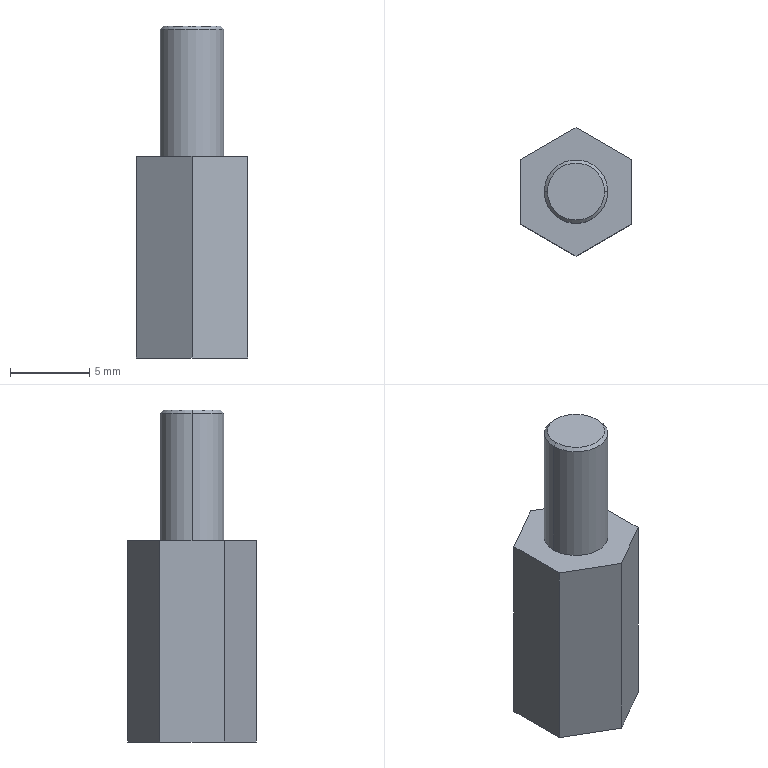Part | STEP file | 49711204_74 | 1 solid | 16 faces | box 7 x 8.09 x 20.9 mm | volume 569.977 mm3 | plane 10 | cylinder 4 | cone 2 | commonest cylinder face diameters 3.2 x2 4 x2
STEP:
#1=CARTESIAN_POINT('',(0.,0.,0.));
#2=DIRECTION('',(0.,0.,1.));
#3=DIRECTION('',(1.,0.,0.));
#4=AXIS2_PLACEMENT_3D('',#1,#2,#3);
#5=CARTESIAN_POINT('',(3.5,-2.024,0.));
#6=VERTEX_POINT('',#5);
#7=CARTESIAN_POINT('',(3.5,2.024,0.));
#8=VERTEX_POINT('',#7);
#9=CARTESIAN_POINT('',(3.5,-2.024,0.));
#10=DIRECTION('',(0.,1.,0.));
#11=VECTOR('',#10,1.);
#12=LINE('',#9,#11);
#13=CARTESIAN_POINT('',(0.,0.,0.));
#14=DIRECTION('',(0.,0.,-1.));
#15=DIRECTION('',(-1.,0.,0.));
#16=AXIS2_PLACEMENT_3D('',#13,#14,#15);
#17=PLANE('',#16);
#18=CARTESIAN_POINT('',(-3.5,-2.024));
#19=DIRECTION('',(0.,1.));
#20=VECTOR('',#19,1.);
#21=LINE('',#18,#20);
#22=(GEOMETRIC_REPRESENTATION_CONTEXT(2)PARAMETRIC_REPRESENTATION_CONTEXT()REPRESENTATION_CONTEXT('',''));
#23=DEFINITIONAL_REPRESENTATION('',(#21),#22);
#24=PCURVE('',#17,#23);
#25=CARTESIAN_POINT('',(3.5,0.,0.));
#26=DIRECTION('',(-1.,0.,0.));
#27=DIRECTION('',(0.,1.,0.));
#28=AXIS2_PLACEMENT_3D('',#25,#26,#27);
#29=PLANE('',#28);
#30=CARTESIAN_POINT('',(-2.024,0.));
#31=DIRECTION('',(1.,0.));
#32=VECTOR('',#31,1.);
#33=LINE('',#30,#32);
#34=(GEOMETRIC_REPRESENTATION_CONTEXT(2)PARAMETRIC_REPRESENTATION_CONTEXT()REPRESENTATION_CONTEXT('',''));
#35=DEFINITIONAL_REPRESENTATION('',(#33),#34);
#36=PCURVE('',#29,#35);
#37=SURFACE_CURVE('',#12,(#24,#36),.PCURVE_S1.);
#38=EDGE_CURVE('',#6,#8,#37,.T.);
#39=ORIENTED_EDGE('',*,*,#38,.F.);
#40=CARTESIAN_POINT('',(0.,-4.045,0.));
#41=VERTEX_POINT('',#40);
#42=CARTESIAN_POINT('',(3.5,-2.024,0.));
#43=DIRECTION('',(-0.866,-0.5,0.));
#44=VECTOR('',#43,1.);
#45=LINE('',#42,#44);
#46=CARTESIAN_POINT('',(-3.5,-2.024));
#47=DIRECTION('',(0.866,-0.5));
#48=VECTOR('',#47,1.);
#49=LINE('',#46,#48);
#50=(GEOMETRIC_REPRESENTATION_CONTEXT(2)PARAMETRIC_REPRESENTATION_CONTEXT()REPRESENTATION_CONTEXT('',''));
#51=DEFINITIONAL_REPRESENTATION('',(#49),#50);
#52=PCURVE('',#17,#51);
#53=CARTESIAN_POINT('',(3.5,-2.024,0.));
#54=DIRECTION('',(0.5,-0.866,0.));
#55=DIRECTION('',(-0.866,-0.5,0.));
#56=AXIS2_PLACEMENT_3D('',#53,#54,#55);
#57=PLANE('',#56);
#58=CARTESIAN_POINT('',(0.,0.));
#59=DIRECTION('',(1.,0.));
#60=VECTOR('',#59,1.);
#61=LINE('',#58,#60);
#62=(GEOMETRIC_REPRESENTATION_CONTEXT(2)PARAMETRIC_REPRESENTATION_CONTEXT()REPRESENTATION_CONTEXT('',''));
#63=DEFINITIONAL_REPRESENTATION('',(#61),#62);
#64=PCURVE('',#57,#63);
#65=SURFACE_CURVE('',#45,(#52,#64),.PCURVE_S1.);
#66=EDGE_CURVE('',#6,#41,#65,.T.);
#67=ORIENTED_EDGE('',*,*,#66,.T.);
#68=CARTESIAN_POINT('',(-3.5,-2.024,0.));
#69=VERTEX_POINT('',#68);
#70=CARTESIAN_POINT('',(-3.5,-2.024,0.));
#71=DIRECTION('',(0.866,-0.5,0.));
#72=VECTOR('',#71,1.);
#73=LINE('',#70,#72);
#74=CARTESIAN_POINT('',(3.5,-2.024));
#75=DIRECTION('',(-0.866,-0.5));
#76=VECTOR('',#75,1.);
#77=LINE('',#74,#76);
#78=(GEOMETRIC_REPRESENTATION_CONTEXT(2)PARAMETRIC_REPRESENTATION_CONTEXT()REPRESENTATION_CONTEXT('',''));
#79=DEFINITIONAL_REPRESENTATION('',(#77),#78);
#80=PCURVE('',#17,#79);
#81=CARTESIAN_POINT('',(-3.5,-2.024,0.));
#82=DIRECTION('',(0.5,0.866,0.));
#83=DIRECTION('',(0.866,-0.5,0.));
#84=AXIS2_PLACEMENT_3D('',#81,#82,#83);
#85=PLANE('',#84);
#86=CARTESIAN_POINT('',(0.,0.));
#87=DIRECTION('',(1.,0.));
#88=VECTOR('',#87,1.);
#89=LINE('',#86,#88);
#90=(GEOMETRIC_REPRESENTATION_CONTEXT(2)PARAMETRIC_REPRESENTATION_CONTEXT()REPRESENTATION_CONTEXT('',''));
#91=DEFINITIONAL_REPRESENTATION('',(#89),#90);
#92=PCURVE('',#85,#91);
#93=SURFACE_CURVE('',#73,(#80,#92),.PCURVE_S1.);
#94=EDGE_CURVE('',#69,#41,#93,.T.);
#95=ORIENTED_EDGE('',*,*,#94,.F.);
#96=CARTESIAN_POINT('',(-3.5,2.024,0.));
#97=VERTEX_POINT('',#96);
#98=CARTESIAN_POINT('',(-3.5,2.024,0.));
#99=DIRECTION('',(0.,-1.,0.));
#100=VECTOR('',#99,1.);
#101=LINE('',#98,#100);
#102=CARTESIAN_POINT('',(3.5,2.024));
#103=DIRECTION('',(0.,-1.));
#104=VECTOR('',#103,1.);
#105=LINE('',#102,#104);
#106=(GEOMETRIC_REPRESENTATION_CONTEXT(2)PARAMETRIC_REPRESENTATION_CONTEXT()REPRESENTATION_CONTEXT('',''));
#107=DEFINITIONAL_REPRESENTATION('',(#105),#106);
#108=PCURVE('',#17,#107);
#109=CARTESIAN_POINT('',(-3.5,0.,0.));
#110=DIRECTION('',(-1.,0.,0.));
#111=DIRECTION('',(0.,1.,0.));
#112=AXIS2_PLACEMENT_3D('',#109,#110,#111);
#113=PLANE('',#112);
#114=CARTESIAN_POINT('',(2.024,0.));
#115=DIRECTION('',(-1.,0.));
#116=VECTOR('',#115,1.);
#117=LINE('',#114,#116);
#118=(GEOMETRIC_REPRESENTATION_CONTEXT(2)PARAMETRIC_REPRESENTATION_CONTEXT()REPRESENTATION_CONTEXT('',''));
#119=DEFINITIONAL_REPRESENTATION('',(#117),#118);
#120=PCURVE('',#113,#119);
#121=SURFACE_CURVE('',#101,(#108,#120),.PCURVE_S1.);
#122=EDGE_CURVE('',#97,#69,#121,.T.);
#123=ORIENTED_EDGE('',*,*,#122,.F.);
#124=CARTESIAN_POINT('',(0.,4.045,0.));
#125=VERTEX_POINT('',#124);
#126=CARTESIAN_POINT('',(-3.5,2.024,0.));
#127=DIRECTION('',(0.866,0.5,0.));
#128=VECTOR('',#127,1.);
#129=LINE('',#126,#128);
#130=CARTESIAN_POINT('',(3.5,2.024));
#131=DIRECTION('',(-0.866,0.5));
#132=VECTOR('',#131,1.);
#133=LINE('',#130,#132);
#134=(GEOMETRIC_REPRESENTATION_CONTEXT(2)PARAMETRIC_REPRESENTATION_CONTEXT()REPRESENTATION_CONTEXT('',''));
#135=DEFINITIONAL_REPRESENTATION('',(#133),#134);
#136=PCURVE('',#17,#135);
#137=CARTESIAN_POINT('',(-3.5,2.024,0.));
#138=DIRECTION('',(-0.5,0.866,0.));
#139=DIRECTION('',(0.866,0.5,0.));
#140=AXIS2_PLACEMENT_3D('',#137,#138,#139);
#141=PLANE('',#140);
#142=CARTESIAN_POINT('',(0.,0.));
#143=DIRECTION('',(1.,0.));
#144=VECTOR('',#143,1.);
#145=LINE('',#142,#144);
#146=(GEOMETRIC_REPRESENTATION_CONTEXT(2)PARAMETRIC_REPRESENTATION_CONTEXT()REPRESENTATION_CONTEXT('',''));
#147=DEFINITIONAL_REPRESENTATION('',(#145),#146);
#148=PCURVE('',#141,#147);
#149=SURFACE_CURVE('',#129,(#136,#148),.PCURVE_S1.);
#150=EDGE_CURVE('',#97,#125,#149,.T.);
#151=ORIENTED_EDGE('',*,*,#150,.T.);
#152=CARTESIAN_POINT('',(3.5,2.024,0.));
#153=DIRECTION('',(-0.866,0.5,0.));
#154=VECTOR('',#153,1.);
#155=LINE('',#152,#154);
#156=CARTESIAN_POINT('',(-3.5,2.024));
#157=DIRECTION('',(0.866,0.5));
#158=VECTOR('',#157,1.);
#159=LINE('',#156,#158);
#160=(GEOMETRIC_REPRESENTATION_CONTEXT(2)PARAMETRIC_REPRESENTATION_CONTEXT()REPRESENTATION_CONTEXT('',''));
#161=DEFINITIONAL_REPRESENTATION('',(#159),#160);
#162=PCURVE('',#17,#161);
#163=CARTESIAN_POINT('',(3.5,2.024,0.));
#164=DIRECTION('',(-0.5,-0.866,0.));
#165=DIRECTION('',(-0.866,0.5,0.));
#166=AXIS2_PLACEMENT_3D('',#163,#164,#165);
#167=PLANE('',#166);
#168=CARTESIAN_POINT('',(0.,0.));
#169=DIRECTION('',(1.,0.));
#170=VECTOR('',#169,1.);
#171=LINE('',#168,#170);
#172=(GEOMETRIC_REPRESENTATION_CONTEXT(2)PARAMETRIC_REPRESENTATION_CONTEXT()REPRESENTATION_CONTEXT('',''));
#173=DEFINITIONAL_REPRESENTATION('',(#171),#172);
#174=PCURVE('',#167,#173);
#175=SURFACE_CURVE('',#155,(#162,#174),.PCURVE_S1.);
#176=EDGE_CURVE('',#8,#125,#175,.T.);
#177=ORIENTED_EDGE('',*,*,#176,.F.);
#178=EDGE_LOOP('',(#39,#67,#95,#123,#151,#177));
#179=FACE_BOUND('',#178,.F.);
#180=CARTESIAN_POINT('',(-2.,0.,0.));
#181=VERTEX_POINT('',#180);
#182=CARTESIAN_POINT('',(2.,0.,0.));
#183=VERTEX_POINT('',#182);
#184=CARTESIAN_POINT('',(0.,0.,0.));
#185=DIRECTION('',(0.,0.,1.));
#186=DIRECTION('',(-1.,0.,0.));
#187=AXIS2_PLACEMENT_3D('',#184,#185,#186);
#188=CIRCLE('',#187,2.);
#189=CARTESIAN_POINT('',(2.,0.));
#190=CARTESIAN_POINT('',(2.,-3.464));
#191=CARTESIAN_POINT('',(-1.,-1.732));
#192=CARTESIAN_POINT('',(-4.,0.));
#193=CARTESIAN_POINT('',(-1.,1.732));
#194=CARTESIAN_POINT('',(2.,3.464));
#195=CARTESIAN_POINT('',(2.,0.));
#196=(BOUNDED_CURVE()B_SPLINE_CURVE(2,(#189,#190,#191,#192,#193,#194,#195),.UNSPECIFIED.,.T.,.F.)B_SPLINE_CURVE_WITH_KNOTS((1,2,2,2,2,1),(-2.094,0.,2.094,4.189,6.283,8.378),.UNSPECIFIED.)CURVE()GEOMETRIC_REPRESENTATION_ITEM()RATIONAL_B_SPLINE_CURVE((1.,0.5,1.,0.5,1.,0.5,1.))REPRESENTATION_ITEM(''));
#197=(GEOMETRIC_REPRESENTATION_CONTEXT(2)PARAMETRIC_REPRESENTATION_CONTEXT()REPRESENTATION_CONTEXT('',''));
#198=DEFINITIONAL_REPRESENTATION('',(#196),#197);
#199=PCURVE('',#17,#198);
#200=CARTESIAN_POINT('',(0.,0.,0.));
#201=DIRECTION('',(0.,0.,1.));
#202=DIRECTION('',(-1.,0.,0.));
#203=AXIS2_PLACEMENT_3D('',#200,#201,#202);
#204=CYLINDRICAL_SURFACE('',#203,2.);
#205=CARTESIAN_POINT('',(0.,0.));
#206=DIRECTION('',(1.,0.));
#207=VECTOR('',#206,1.);
#208=LINE('',#205,#207);
#209=(GEOMETRIC_REPRESENTATION_CONTEXT(2)PARAMETRIC_REPRESENTATION_CONTEXT()REPRESENTATION_CONTEXT('',''));
#210=DEFINITIONAL_REPRESENTATION('',(#208),#209);
#211=PCURVE('',#204,#210);
#212=SURFACE_CURVE('',#188,(#199,#211),.PCURVE_S1.);
#213=EDGE_CURVE('',#181,#183,#212,.T.);
#214=ORIENTED_EDGE('',*,*,#213,.T.);
#215=CARTESIAN_POINT('',(0.,0.,0.));
#216=DIRECTION('',(0.,0.,1.));
#217=DIRECTION('',(1.,0.,0.));
#218=AXIS2_PLACEMENT_3D('',#215,#216,#217);
#219=CIRCLE('',#218,2.);
#220=CARTESIAN_POINT('',(-2.,0.));
#221=CARTESIAN_POINT('',(-2.,3.464));
#222=CARTESIAN_POINT('',(1.,1.732));
#223=CARTESIAN_POINT('',(4.,0.));
#224=CARTESIAN_POINT('',(1.,-1.732));
#225=CARTESIAN_POINT('',(-2.,-3.464));
#226=CARTESIAN_POINT('',(-2.,0.));
#227=(BOUNDED_CURVE()B_SPLINE_CURVE(2,(#220,#221,#222,#223,#224,#225,#226),.UNSPECIFIED.,.T.,.F.)B_SPLINE_CURVE_WITH_KNOTS((1,2,2,2,2,1),(-2.094,0.,2.094,4.189,6.283,8.378),.UNSPECIFIED.)CURVE()GEOMETRIC_REPRESENTATION_ITEM()RATIONAL_B_SPLINE_CURVE((1.,0.5,1.,0.5,1.,0.5,1.))REPRESENTATION_ITEM(''));
#228=(GEOMETRIC_REPRESENTATION_CONTEXT(2)PARAMETRIC_REPRESENTATION_CONTEXT()REPRESENTATION_CONTEXT('',''));
#229=DEFINITIONAL_REPRESENTATION('',(#227),#228);
#230=PCURVE('',#17,#229);
#231=CARTESIAN_POINT('',(0.,0.,0.));
#232=DIRECTION('',(0.,0.,1.));
#233=DIRECTION('',(-1.,0.,0.));
#234=AXIS2_PLACEMENT_3D('',#231,#232,#233);
#235=CYLINDRICAL_SURFACE('',#234,2.);
#236=CARTESIAN_POINT('',(3.142,0.));
#237=DIRECTION('',(1.,0.));
#238=VECTOR('',#237,1.);
#239=LINE('',#236,#238);
#240=(GEOMETRIC_REPRESENTATION_CONTEXT(2)PARAMETRIC_REPRESENTATION_CONTEXT()REPRESENTATION_CONTEXT('',''));
#241=DEFINITIONAL_REPRESENTATION('',(#239),#240);
#242=PCURVE('',#235,#241);
#243=SURFACE_CURVE('',#219,(#230,#242),.PCURVE_S1.);
#244=EDGE_CURVE('',#183,#181,#243,.T.);
#245=ORIENTED_EDGE('',*,*,#244,.T.);
#246=EDGE_LOOP('',(#214,#245));
#247=FACE_BOUND('',#246,.F.);
#248=ADVANCED_FACE('',(#179,#247),#17,.F.);
#249=CARTESIAN_POINT('',(3.5,2.024,-12.7));
#250=VERTEX_POINT('',#249);
#251=CARTESIAN_POINT('',(3.5,-2.024,-12.7));
#252=VERTEX_POINT('',#251);
#253=CARTESIAN_POINT('',(3.5,2.024,-12.7));
#254=DIRECTION('',(0.,-1.,0.));
#255=VECTOR('',#254,1.);
#256=LINE('',#253,#255);
#257=CARTESIAN_POINT('',(2.024,12.7));
#258=DIRECTION('',(-1.,0.));
#259=VECTOR('',#258,1.);
#260=LINE('',#257,#259);
#261=(GEOMETRIC_REPRESENTATION_CONTEXT(2)PARAMETRIC_REPRESENTATION_CONTEXT()REPRESENTATION_CONTEXT('',''));
#262=DEFINITIONAL_REPRESENTATION('',(#260),#261);
#263=PCURVE('',#29,#262);
#264=CARTESIAN_POINT('',(0.,0.,-12.7));
#265=DIRECTION('',(0.,0.,-1.));
#266=DIRECTION('',(-1.,0.,0.));
#267=AXIS2_PLACEMENT_3D('',#264,#265,#266);
#268=PLANE('',#267);
#269=CARTESIAN_POINT('',(-3.5,2.024));
#270=DIRECTION('',(0.,-1.));
#271=VECTOR('',#270,1.);
#272=LINE('',#269,#271);
#273=(GEOMETRIC_REPRESENTATION_CONTEXT(2)PARAMETRIC_REPRESENTATION_CONTEXT()REPRESENTATION_CONTEXT('',''));
#274=DEFINITIONAL_REPRESENTATION('',(#272),#273);
#275=PCURVE('',#268,#274);
#276=SURFACE_CURVE('',#256,(#263,#275),.PCURVE_S1.);
#277=EDGE_CURVE('',#250,#252,#276,.T.);
#278=ORIENTED_EDGE('',*,*,#277,.T.);
#279=CARTESIAN_POINT('',(3.5,-2.024,0.));
#280=DIRECTION('',(0.,0.,-1.));
#281=VECTOR('',#280,1.);
#282=LINE('',#279,#281);
#283=CARTESIAN_POINT('',(-2.024,0.));
#284=DIRECTION('',(0.,1.));
#285=VECTOR('',#284,1.);
#286=LINE('',#283,#285);
#287=(GEOMETRIC_REPRESENTATION_CONTEXT(2)PARAMETRIC_REPRESENTATION_CONTEXT()REPRESENTATION_CONTEXT('',''));
#288=DEFINITIONAL_REPRESENTATION('',(#286),#287);
#289=PCURVE('',#29,#288);
#290=CARTESIAN_POINT('',(0.,0.));
#291=DIRECTION('',(0.,1.));
#292=VECTOR('',#291,1.);
#293=LINE('',#290,#292);
#294=(GEOMETRIC_REPRESENTATION_CONTEXT(2)PARAMETRIC_REPRESENTATION_CONTEXT()REPRESENTATION_CONTEXT('',''));
#295=DEFINITIONAL_REPRESENTATION('',(#293),#294);
#296=PCURVE('',#57,#295);
#297=SURFACE_CURVE('',#282,(#289,#296),.PCURVE_S1.);
#298=EDGE_CURVE('',#6,#252,#297,.T.);
#299=ORIENTED_EDGE('',*,*,#298,.F.);
#300=ORIENTED_EDGE('',*,*,#38,.T.);
#301=CARTESIAN_POINT('',(3.5,2.024,0.));
#302=DIRECTION('',(0.,0.,-1.));
#303=VECTOR('',#302,1.);
#304=LINE('',#301,#303);
#305=CARTESIAN_POINT('',(2.024,0.));
#306=DIRECTION('',(0.,1.));
#307=VECTOR('',#306,1.);
#308=LINE('',#305,#307);
#309=(GEOMETRIC_REPRESENTATION_CONTEXT(2)PARAMETRIC_REPRESENTATION_CONTEXT()REPRESENTATION_CONTEXT('',''));
#310=DEFINITIONAL_REPRESENTATION('',(#308),#309);
#311=PCURVE('',#29,#310);
#312=CARTESIAN_POINT('',(0.,0.));
#313=DIRECTION('',(0.,1.));
#314=VECTOR('',#313,1.);
#315=LINE('',#312,#314);
#316=(GEOMETRIC_REPRESENTATION_CONTEXT(2)PARAMETRIC_REPRESENTATION_CONTEXT()REPRESENTATION_CONTEXT('',''));
#317=DEFINITIONAL_REPRESENTATION('',(#315),#316);
#318=PCURVE('',#167,#317);
#319=SURFACE_CURVE('',#304,(#311,#318),.PCURVE_S1.);
#320=EDGE_CURVE('',#8,#250,#319,.T.);
#321=ORIENTED_EDGE('',*,*,#320,.T.);
#322=EDGE_LOOP('',(#278,#299,#300,#321));
#323=FACE_BOUND('',#322,.F.);
#324=ADVANCED_FACE('',(#323),#29,.F.);
#325=CARTESIAN_POINT('',(-3.5,-2.024,-12.7));
#326=VERTEX_POINT('',#325);
#327=CARTESIAN_POINT('',(0.,-4.045,-12.7));
#328=VERTEX_POINT('',#327);
#329=CARTESIAN_POINT('',(-3.5,-2.024,-12.7));
#330=DIRECTION('',(0.866,-0.5,0.));
#331=VECTOR('',#330,1.);
#332=LINE('',#329,#331);
#333=CARTESIAN_POINT('',(3.5,-2.024));
#334=DIRECTION('',(-0.866,-0.5));
#335=VECTOR('',#334,1.);
#336=LINE('',#333,#335);
#337=(GEOMETRIC_REPRESENTATION_CONTEXT(2)PARAMETRIC_REPRESENTATION_CONTEXT()REPRESENTATION_CONTEXT('',''));
#338=DEFINITIONAL_REPRESENTATION('',(#336),#337);
#339=PCURVE('',#268,#338);
#340=CARTESIAN_POINT('',(0.,12.7));
#341=DIRECTION('',(1.,0.));
#342=VECTOR('',#341,1.);
#343=LINE('',#340,#342);
#344=(GEOMETRIC_REPRESENTATION_CONTEXT(2)PARAMETRIC_REPRESENTATION_CONTEXT()REPRESENTATION_CONTEXT('',''));
#345=DEFINITIONAL_REPRESENTATION('',(#343),#344);
#346=PCURVE('',#85,#345);
#347=SURFACE_CURVE('',#332,(#339,#346),.PCURVE_S1.);
#348=EDGE_CURVE('',#326,#328,#347,.T.);
#349=ORIENTED_EDGE('',*,*,#348,.T.);
#350=CARTESIAN_POINT('',(3.5,-2.024,-12.7));
#351=DIRECTION('',(-0.866,-0.5,0.));
#352=VECTOR('',#351,1.);
#353=LINE('',#350,#352);
#354=CARTESIAN_POINT('',(-3.5,-2.024));
#355=DIRECTION('',(0.866,-0.5));
#356=VECTOR('',#355,1.);
#357=LINE('',#354,#356);
#358=(GEOMETRIC_REPRESENTATION_CONTEXT(2)PARAMETRIC_REPRESENTATION_CONTEXT()REPRESENTATION_CONTEXT('',''));
#359=DEFINITIONAL_REPRESENTATION('',(#357),#358);
#360=PCURVE('',#268,#359);
#361=CARTESIAN_POINT('',(0.,12.7));
#362=DIRECTION('',(1.,0.));
#363=VECTOR('',#362,1.);
#364=LINE('',#361,#363);
#365=(GEOMETRIC_REPRESENTATION_CONTEXT(2)PARAMETRIC_REPRESENTATION_CONTEXT()REPRESENTATION_CONTEXT('',''));
#366=DEFINITIONAL_REPRESENTATION('',(#364),#365);
#367=PCURVE('',#57,#366);
#368=SURFACE_CURVE('',#353,(#360,#367),.PCURVE_S1.);
#369=EDGE_CURVE('',#252,#328,#368,.T.);
#370=ORIENTED_EDGE('',*,*,#369,.F.);
#371=ORIENTED_EDGE('',*,*,#277,.F.);
#372=CARTESIAN_POINT('',(0.,4.045,-12.7));
#373=VERTEX_POINT('',#372);
#374=CARTESIAN_POINT('',(3.5,2.024,-12.7));
#375=DIRECTION('',(-0.866,0.5,0.));
#376=VECTOR('',#375,1.);
#377=LINE('',#374,#376);
#378=CARTESIAN_POINT('',(-3.5,2.024));
#379=DIRECTION('',(0.866,0.5));
#380=VECTOR('',#379,1.);
#381=LINE('',#378,#380);
#382=(GEOMETRIC_REPRESENTATION_CONTEXT(2)PARAMETRIC_REPRESENTATION_CONTEXT()REPRESENTATION_CONTEXT('',''));
#383=DEFINITIONAL_REPRESENTATION('',(#381),#382);
#384=PCURVE('',#268,#383);
#385=CARTESIAN_POINT('',(0.,12.7));
#386=DIRECTION('',(1.,0.));
#387=VECTOR('',#386,1.);
#388=LINE('',#385,#387);
#389=(GEOMETRIC_REPRESENTATION_CONTEXT(2)PARAMETRIC_REPRESENTATION_CONTEXT()REPRESENTATION_CONTEXT('',''));
#390=DEFINITIONAL_REPRESENTATION('',(#388),#389);
#391=PCURVE('',#167,#390);
#392=SURFACE_CURVE('',#377,(#384,#391),.PCURVE_S1.);
#393=EDGE_CURVE('',#250,#373,#392,.T.);
#394=ORIENTED_EDGE('',*,*,#393,.T.);
#395=CARTESIAN_POINT('',(-3.5,2.024,-12.7));
#396=VERTEX_POINT('',#395);
#397=CARTESIAN_POINT('',(-3.5,2.024,-12.7));
#398=DIRECTION('',(0.866,0.5,0.));
#399=VECTOR('',#398,1.);
#400=LINE('',#397,#399);
#401=CARTESIAN_POINT('',(3.5,2.024));
#402=DIRECTION('',(-0.866,0.5));
#403=VECTOR('',#402,1.);
#404=LINE('',#401,#403);
#405=(GEOMETRIC_REPRESENTATION_CONTEXT(2)PARAMETRIC_REPRESENTATION_CONTEXT()REPRESENTATION_CONTEXT('',''));
#406=DEFINITIONAL_REPRESENTATION('',(#404),#405);
#407=PCURVE('',#268,#406);
#408=CARTESIAN_POINT('',(0.,12.7));
#409=DIRECTION('',(1.,0.));
#410=VECTOR('',#409,1.);
#411=LINE('',#408,#410);
#412=(GEOMETRIC_REPRESENTATION_CONTEXT(2)PARAMETRIC_REPRESENTATION_CONTEXT()REPRESENTATION_CONTEXT('',''));
#413=DEFINITIONAL_REPRESENTATION('',(#411),#412);
#414=PCURVE('',#141,#413);
#415=SURFACE_CURVE('',#400,(#407,#414),.PCURVE_S1.);
#416=EDGE_CURVE('',#396,#373,#415,.T.);
#417=ORIENTED_EDGE('',*,*,#416,.F.);
#418=CARTESIAN_POINT('',(-3.5,-2.024,-12.7));
#419=DIRECTION('',(0.,1.,0.));
#420=VECTOR('',#419,1.);
#421=LINE('',#418,#420);
#422=CARTESIAN_POINT('',(3.5,-2.024));
#423=DIRECTION('',(0.,1.));
#424=VECTOR('',#423,1.);
#425=LINE('',#422,#424);
#426=(GEOMETRIC_REPRESENTATION_CONTEXT(2)PARAMETRIC_REPRESENTATION_CONTEXT()REPRESENTATION_CONTEXT('',''));
#427=DEFINITIONAL_REPRESENTATION('',(#425),#426);
#428=PCURVE('',#268,#427);
#429=CARTESIAN_POINT('',(-2.024,12.7));
#430=DIRECTION('',(1.,0.));
#431=VECTOR('',#430,1.);
#432=LINE('',#429,#431);
#433=(GEOMETRIC_REPRESENTATION_CONTEXT(2)PARAMETRIC_REPRESENTATION_CONTEXT()REPRESENTATION_CONTEXT('',''));
#434=DEFINITIONAL_REPRESENTATION('',(#432),#433);
#435=PCURVE('',#113,#434);
#436=SURFACE_CURVE('',#421,(#428,#435),.PCURVE_S1.);
#437=EDGE_CURVE('',#326,#396,#436,.T.);
#438=ORIENTED_EDGE('',*,*,#437,.F.);
#439=EDGE_LOOP('',(#349,#370,#371,#394,#417,#438));
#440=FACE_BOUND('',#439,.F.);
#441=CARTESIAN_POINT('',(1.6,0.,-12.7));
#442=VERTEX_POINT('',#441);
#443=CARTESIAN_POINT('',(-1.6,0.,-12.7));
#444=VERTEX_POINT('',#443);
#445=CARTESIAN_POINT('',(0.,0.,-12.7));
#446=DIRECTION('',(0.,0.,-1.));
#447=DIRECTION('',(1.,0.,0.));
#448=AXIS2_PLACEMENT_3D('',#445,#446,#447);
#449=CIRCLE('',#448,1.6);
#450=CARTESIAN_POINT('',(0.,0.));
#451=DIRECTION('',(-1.,0.));
#452=AXIS2_PLACEMENT_2D('',#450,#451);
#453=CIRCLE('',#452,1.6);
#454=(GEOMETRIC_REPRESENTATION_CONTEXT(2)PARAMETRIC_REPRESENTATION_CONTEXT()REPRESENTATION_CONTEXT('',''));
#455=DEFINITIONAL_REPRESENTATION('',(#453),#454);
#456=PCURVE('',#268,#455);
#457=CARTESIAN_POINT('',(0.,0.,-12.7));
#458=DIRECTION('',(0.,0.,-1.));
#459=DIRECTION('',(1.,0.,0.));
#460=AXIS2_PLACEMENT_3D('',#457,#458,#459);
#461=CYLINDRICAL_SURFACE('',#460,1.6);
#462=CARTESIAN_POINT('',(0.,0.));
#463=DIRECTION('',(1.,0.));
#464=VECTOR('',#463,1.);
#465=LINE('',#462,#464);
#466=(GEOMETRIC_REPRESENTATION_CONTEXT(2)PARAMETRIC_REPRESENTATION_CONTEXT()REPRESENTATION_CONTEXT('',''));
#467=DEFINITIONAL_REPRESENTATION('',(#465),#466);
#468=PCURVE('',#461,#467);
#469=SURFACE_CURVE('',#449,(#456,#468),.PCURVE_S1.);
#470=EDGE_CURVE('',#442,#444,#469,.T.);
#471=ORIENTED_EDGE('',*,*,#470,.T.);
#472=CARTESIAN_POINT('',(0.,0.,-12.7));
#473=DIRECTION('',(0.,0.,-1.));
#474=DIRECTION('',(-1.,0.,0.));
#475=AXIS2_PLACEMENT_3D('',#472,#473,#474);
#476=CIRCLE('',#475,1.6);
#477=CARTESIAN_POINT('',(0.,0.));
#478=DIRECTION('',(1.,0.));
#479=AXIS2_PLACEMENT_2D('',#477,#478);
#480=CIRCLE('',#479,1.6);
#481=(GEOMETRIC_REPRESENTATION_CONTEXT(2)PARAMETRIC_REPRESENTATION_CONTEXT()REPRESENTATION_CONTEXT('',''));
#482=DEFINITIONAL_REPRESENTATION('',(#480),#481);
#483=PCURVE('',#268,#482);
#484=CARTESIAN_POINT('',(0.,0.,-12.7));
#485=DIRECTION('',(0.,0.,-1.));
#486=DIRECTION('',(1.,0.,0.));
#487=AXIS2_PLACEMENT_3D('',#484,#485,#486);
#488=CYLINDRICAL_SURFACE('',#487,1.6);
#489=CARTESIAN_POINT('',(3.142,0.));
#490=DIRECTION('',(1.,0.));
#491=VECTOR('',#490,1.);
#492=LINE('',#489,#491);
#493=(GEOMETRIC_REPRESENTATION_CONTEXT(2)PARAMETRIC_REPRESENTATION_CONTEXT()REPRESENTATION_CONTEXT('',''));
#494=DEFINITIONAL_REPRESENTATION('',(#492),#493);
#495=PCURVE('',#488,#494);
#496=SURFACE_CURVE('',#476,(#483,#495),.PCURVE_S1.);
#497=EDGE_CURVE('',#444,#442,#496,.T.);
#498=ORIENTED_EDGE('',*,*,#497,.T.);
#499=EDGE_LOOP('',(#471,#498));
#500=FACE_BOUND('',#499,.F.);
#501=ADVANCED_FACE('',(#440,#500),#268,.T.);
#502=CARTESIAN_POINT('',(0.,-4.045,0.));
#503=DIRECTION('',(0.,0.,-1.));
#504=VECTOR('',#503,1.);
#505=LINE('',#502,#504);
#506=CARTESIAN_POINT('',(4.041,0.));
#507=DIRECTION('',(0.,1.));
#508=VECTOR('',#507,1.);
#509=LINE('',#506,#508);
#510=(GEOMETRIC_REPRESENTATION_CONTEXT(2)PARAMETRIC_REPRESENTATION_CONTEXT()REPRESENTATION_CONTEXT('',''));
#511=DEFINITIONAL_REPRESENTATION('',(#509),#510);
#512=PCURVE('',#85,#511);
#513=CARTESIAN_POINT('',(4.041,0.));
#514=DIRECTION('',(0.,1.));
#515=VECTOR('',#514,1.);
#516=LINE('',#513,#515);
#517=(GEOMETRIC_REPRESENTATION_CONTEXT(2)PARAMETRIC_REPRESENTATION_CONTEXT()REPRESENTATION_CONTEXT('',''));
#518=DEFINITIONAL_REPRESENTATION('',(#516),#517);
#519=PCURVE('',#57,#518);
#520=SURFACE_CURVE('',#505,(#512,#519),.PCURVE_S1.);
#521=EDGE_CURVE('',#41,#328,#520,.T.);
#522=ORIENTED_EDGE('',*,*,#521,.T.);
#523=ORIENTED_EDGE('',*,*,#348,.F.);
#524=CARTESIAN_POINT('',(-3.5,-2.024,0.));
#525=DIRECTION('',(0.,0.,-1.));
#526=VECTOR('',#525,1.);
#527=LINE('',#524,#526);
#528=CARTESIAN_POINT('',(0.,0.));
#529=DIRECTION('',(0.,1.));
#530=VECTOR('',#529,1.);
#531=LINE('',#528,#530);
#532=(GEOMETRIC_REPRESENTATION_CONTEXT(2)PARAMETRIC_REPRESENTATION_CONTEXT()REPRESENTATION_CONTEXT('',''));
#533=DEFINITIONAL_REPRESENTATION('',(#531),#532);
#534=PCURVE('',#85,#533);
#535=CARTESIAN_POINT('',(-2.024,0.));
#536=DIRECTION('',(0.,1.));
#537=VECTOR('',#536,1.);
#538=LINE('',#535,#537);
#539=(GEOMETRIC_REPRESENTATION_CONTEXT(2)PARAMETRIC_REPRESENTATION_CONTEXT()REPRESENTATION_CONTEXT('',''));
#540=DEFINITIONAL_REPRESENTATION('',(#538),#539);
#541=PCURVE('',#113,#540);
#542=SURFACE_CURVE('',#527,(#534,#541),.PCURVE_S1.);
#543=EDGE_CURVE('',#69,#326,#542,.T.);
#544=ORIENTED_EDGE('',*,*,#543,.F.);
#545=ORIENTED_EDGE('',*,*,#94,.T.);
#546=EDGE_LOOP('',(#522,#523,#544,#545));
#547=FACE_BOUND('',#546,.F.);
#548=ADVANCED_FACE('',(#547),#85,.F.);
#549=ORIENTED_EDGE('',*,*,#521,.F.);
#550=ORIENTED_EDGE('',*,*,#66,.F.);
#551=ORIENTED_EDGE('',*,*,#298,.T.);
#552=ORIENTED_EDGE('',*,*,#369,.T.);
#553=EDGE_LOOP('',(#549,#550,#551,#552));
#554=FACE_BOUND('',#553,.F.);
#555=ADVANCED_FACE('',(#554),#57,.T.);
#556=ORIENTED_EDGE('',*,*,#122,.T.);
#557=ORIENTED_EDGE('',*,*,#543,.T.);
#558=ORIENTED_EDGE('',*,*,#437,.T.);
#559=CARTESIAN_POINT('',(-3.5,2.024,0.));
#560=DIRECTION('',(0.,0.,-1.));
#561=VECTOR('',#560,1.);
#562=LINE('',#559,#561);
#563=CARTESIAN_POINT('',(2.024,0.));
#564=DIRECTION('',(0.,1.));
#565=VECTOR('',#564,1.);
#566=LINE('',#563,#565);
#567=(GEOMETRIC_REPRESENTATION_CONTEXT(2)PARAMETRIC_REPRESENTATION_CONTEXT()REPRESENTATION_CONTEXT('',''));
#568=DEFINITIONAL_REPRESENTATION('',(#566),#567);
#569=PCURVE('',#113,#568);
#570=CARTESIAN_POINT('',(0.,0.));
#571=DIRECTION('',(0.,1.));
#572=VECTOR('',#571,1.);
#573=LINE('',#570,#572);
#574=(GEOMETRIC_REPRESENTATION_CONTEXT(2)PARAMETRIC_REPRESENTATION_CONTEXT()REPRESENTATION_CONTEXT('',''));
#575=DEFINITIONAL_REPRESENTATION('',(#573),#574);
#576=PCURVE('',#141,#575);
#577=SURFACE_CURVE('',#562,(#569,#576),.PCURVE_S1.);
#578=EDGE_CURVE('',#97,#396,#577,.T.);
#579=ORIENTED_EDGE('',*,*,#578,.F.);
#580=EDGE_LOOP('',(#556,#557,#558,#579));
#581=FACE_BOUND('',#580,.F.);
#582=ADVANCED_FACE('',(#581),#113,.T.);
#583=CARTESIAN_POINT('',(0.,4.045,0.));
#584=DIRECTION('',(0.,0.,-1.));
#585=VECTOR('',#584,1.);
#586=LINE('',#583,#585);
#587=CARTESIAN_POINT('',(4.041,0.));
#588=DIRECTION('',(0.,1.));
#589=VECTOR('',#588,1.);
#590=LINE('',#587,#589);
#591=(GEOMETRIC_REPRESENTATION_CONTEXT(2)PARAMETRIC_REPRESENTATION_CONTEXT()REPRESENTATION_CONTEXT('',''));
#592=DEFINITIONAL_REPRESENTATION('',(#590),#591);
#593=PCURVE('',#141,#592);
#594=CARTESIAN_POINT('',(4.041,0.));
#595=DIRECTION('',(0.,1.));
#596=VECTOR('',#595,1.);
#597=LINE('',#594,#596);
#598=(GEOMETRIC_REPRESENTATION_CONTEXT(2)PARAMETRIC_REPRESENTATION_CONTEXT()REPRESENTATION_CONTEXT('',''));
#599=DEFINITIONAL_REPRESENTATION('',(#597),#598);
#600=PCURVE('',#167,#599);
#601=SURFACE_CURVE('',#586,(#593,#600),.PCURVE_S1.);
#602=EDGE_CURVE('',#125,#373,#601,.T.);
#603=ORIENTED_EDGE('',*,*,#602,.F.);
#604=ORIENTED_EDGE('',*,*,#150,.F.);
#605=ORIENTED_EDGE('',*,*,#578,.T.);
#606=ORIENTED_EDGE('',*,*,#416,.T.);
#607=EDGE_LOOP('',(#603,#604,#605,#606));
#608=FACE_BOUND('',#607,.F.);
#609=ADVANCED_FACE('',(#608),#141,.T.);
#610=ORIENTED_EDGE('',*,*,#602,.T.);
#611=ORIENTED_EDGE('',*,*,#393,.F.);
#612=ORIENTED_EDGE('',*,*,#320,.F.);
#613=ORIENTED_EDGE('',*,*,#176,.T.);
#614=EDGE_LOOP('',(#610,#611,#612,#613));
#615=FACE_BOUND('',#614,.F.);
#616=ADVANCED_FACE('',(#615),#167,.F.);
#617=ORIENTED_EDGE('',*,*,#470,.F.);
#618=CARTESIAN_POINT('',(1.6,0.,-3.7));
#619=VERTEX_POINT('',#618);
#620=CARTESIAN_POINT('',(1.6,0.,-12.7));
#621=DIRECTION('',(0.,0.,1.));
#622=VECTOR('',#621,1.);
#623=LINE('',#620,#622);
#624=CARTESIAN_POINT('',(0.,0.));
#625=DIRECTION('',(0.,-1.));
#626=VECTOR('',#625,1.);
#627=LINE('',#624,#626);
#628=(GEOMETRIC_REPRESENTATION_CONTEXT(2)PARAMETRIC_REPRESENTATION_CONTEXT()REPRESENTATION_CONTEXT('',''));
#629=DEFINITIONAL_REPRESENTATION('',(#627),#628);
#630=PCURVE('',#461,#629);
#631=CARTESIAN_POINT('',(6.283,0.));
#632=DIRECTION('',(0.,-1.));
#633=VECTOR('',#632,1.);
#634=LINE('',#631,#633);
#635=(GEOMETRIC_REPRESENTATION_CONTEXT(2)PARAMETRIC_REPRESENTATION_CONTEXT()REPRESENTATION_CONTEXT('',''));
#636=DEFINITIONAL_REPRESENTATION('',(#634),#635);
#637=PCURVE('',#488,#636);
#638=SURFACE_CURVE('',#623,(#630,#637),.PCURVE_S1.);
#639=EDGE_CURVE('',#442,#619,#638,.T.);
#640=ORIENTED_EDGE('',*,*,#639,.T.);
#641=CARTESIAN_POINT('',(-1.6,0.,-3.7));
#642=VERTEX_POINT('',#641);
#643=CARTESIAN_POINT('',(0.,0.,-3.7));
#644=DIRECTION('',(0.,0.,-1.));
#645=DIRECTION('',(1.,0.,0.));
#646=AXIS2_PLACEMENT_3D('',#643,#644,#645);
#647=CIRCLE('',#646,1.6);
#648=CARTESIAN_POINT('',(0.,-9.));
#649=DIRECTION('',(1.,0.));
#650=VECTOR('',#649,1.);
#651=LINE('',#648,#650);
#652=(GEOMETRIC_REPRESENTATION_CONTEXT(2)PARAMETRIC_REPRESENTATION_CONTEXT()REPRESENTATION_CONTEXT('',''));
#653=DEFINITIONAL_REPRESENTATION('',(#651),#652);
#654=PCURVE('',#461,#653);
#655=CARTESIAN_POINT('',(0.,0.,-3.7));
#656=DIRECTION('',(0.,0.,-1.));
#657=DIRECTION('',(1.,0.,0.));
#658=AXIS2_PLACEMENT_3D('',#655,#656,#657);
#659=PLANE('',#658);
#660=CARTESIAN_POINT('',(0.,0.));
#661=DIRECTION('',(1.,0.));
#662=AXIS2_PLACEMENT_2D('',#660,#661);
#663=CIRCLE('',#662,1.6);
#664=(GEOMETRIC_REPRESENTATION_CONTEXT(2)PARAMETRIC_REPRESENTATION_CONTEXT()REPRESENTATION_CONTEXT('',''));
#665=DEFINITIONAL_REPRESENTATION('',(#663),#664);
#666=PCURVE('',#659,#665);
#667=SURFACE_CURVE('',#647,(#654,#666),.PCURVE_S1.);
#668=EDGE_CURVE('',#619,#642,#667,.T.);
#669=ORIENTED_EDGE('',*,*,#668,.T.);
#670=CARTESIAN_POINT('',(-1.6,0.,-12.7));
#671=DIRECTION('',(0.,0.,1.));
#672=VECTOR('',#671,1.);
#673=LINE('',#670,#672);
#674=CARTESIAN_POINT('',(3.142,0.));
#675=DIRECTION('',(0.,-1.));
#676=VECTOR('',#675,1.);
#677=LINE('',#674,#676);
#678=(GEOMETRIC_REPRESENTATION_CONTEXT(2)PARAMETRIC_REPRESENTATION_CONTEXT()REPRESENTATION_CONTEXT('',''));
#679=DEFINITIONAL_REPRESENTATION('',(#677),#678);
#680=PCURVE('',#461,#679);
#681=CARTESIAN_POINT('',(3.142,0.));
#682=DIRECTION('',(0.,-1.));
#683=VECTOR('',#682,1.);
#684=LINE('',#681,#683);
#685=(GEOMETRIC_REPRESENTATION_CONTEXT(2)PARAMETRIC_REPRESENTATION_CONTEXT()REPRESENTATION_CONTEXT('',''));
#686=DEFINITIONAL_REPRESENTATION('',(#684),#685);
#687=PCURVE('',#488,#686);
#688=SURFACE_CURVE('',#673,(#680,#687),.PCURVE_S1.);
#689=EDGE_CURVE('',#444,#642,#688,.T.);
#690=ORIENTED_EDGE('',*,*,#689,.F.);
#691=EDGE_LOOP('',(#617,#640,#669,#690));
#692=FACE_BOUND('',#691,.F.);
#693=ADVANCED_FACE('',(#692),#461,.F.);
#694=ORIENTED_EDGE('',*,*,#497,.F.);
#695=ORIENTED_EDGE('',*,*,#689,.T.);
#696=CARTESIAN_POINT('',(0.,0.,-3.7));
#697=DIRECTION('',(0.,0.,-1.));
#698=DIRECTION('',(-1.,0.,0.));
#699=AXIS2_PLACEMENT_3D('',#696,#697,#698);
#700=CIRCLE('',#699,1.6);
#701=CARTESIAN_POINT('',(3.142,-9.));
#702=DIRECTION('',(1.,0.));
#703=VECTOR('',#702,1.);
#704=LINE('',#701,#703);
#705=(GEOMETRIC_REPRESENTATION_CONTEXT(2)PARAMETRIC_REPRESENTATION_CONTEXT()REPRESENTATION_CONTEXT('',''));
#706=DEFINITIONAL_REPRESENTATION('',(#704),#705);
#707=PCURVE('',#488,#706);
#708=CARTESIAN_POINT('',(0.,0.));
#709=DIRECTION('',(-1.,0.));
#710=AXIS2_PLACEMENT_2D('',#708,#709);
#711=CIRCLE('',#710,1.6);
#712=(GEOMETRIC_REPRESENTATION_CONTEXT(2)PARAMETRIC_REPRESENTATION_CONTEXT()REPRESENTATION_CONTEXT('',''));
#713=DEFINITIONAL_REPRESENTATION('',(#711),#712);
#714=PCURVE('',#659,#713);
#715=SURFACE_CURVE('',#700,(#707,#714),.PCURVE_S1.);
#716=EDGE_CURVE('',#642,#619,#715,.T.);
#717=ORIENTED_EDGE('',*,*,#716,.T.);
#718=ORIENTED_EDGE('',*,*,#639,.F.);
#719=EDGE_LOOP('',(#694,#695,#717,#718));
#720=FACE_BOUND('',#719,.F.);
#721=ADVANCED_FACE('',(#720),#488,.F.);
#722=ORIENTED_EDGE('',*,*,#668,.F.);
#723=ORIENTED_EDGE('',*,*,#716,.F.);
#724=EDGE_LOOP('',(#722,#723));
#725=FACE_BOUND('',#724,.F.);
#726=ADVANCED_FACE('',(#725),#659,.T.);
#727=CARTESIAN_POINT('',(2.,0.,8.));
#728=VERTEX_POINT('',#727);
#729=CARTESIAN_POINT('',(2.,0.,0.));
#730=DIRECTION('',(0.,0.,1.));
#731=VECTOR('',#730,1.);
#732=LINE('',#729,#731);
#733=CARTESIAN_POINT('',(3.142,0.));
#734=DIRECTION('',(0.,1.));
#735=VECTOR('',#734,1.);
#736=LINE('',#733,#735);
#737=(GEOMETRIC_REPRESENTATION_CONTEXT(2)PARAMETRIC_REPRESENTATION_CONTEXT()REPRESENTATION_CONTEXT('',''));
#738=DEFINITIONAL_REPRESENTATION('',(#736),#737);
#739=PCURVE('',#204,#738);
#740=CARTESIAN_POINT('',(3.142,0.));
#741=DIRECTION('',(0.,1.));
#742=VECTOR('',#741,1.);
#743=LINE('',#740,#742);
#744=(GEOMETRIC_REPRESENTATION_CONTEXT(2)PARAMETRIC_REPRESENTATION_CONTEXT()REPRESENTATION_CONTEXT('',''));
#745=DEFINITIONAL_REPRESENTATION('',(#743),#744);
#746=PCURVE('',#235,#745);
#747=SURFACE_CURVE('',#732,(#739,#746),.PCURVE_S1.);
#748=EDGE_CURVE('',#183,#728,#747,.T.);
#749=ORIENTED_EDGE('',*,*,#748,.T.);
#750=CARTESIAN_POINT('',(-2.,0.,8.));
#751=VERTEX_POINT('',#750);
#752=CARTESIAN_POINT('',(0.,0.,8.));
#753=DIRECTION('',(0.,0.,1.));
#754=DIRECTION('',(-1.,0.,0.));
#755=AXIS2_PLACEMENT_3D('',#752,#753,#754);
#756=CIRCLE('',#755,2.);
#757=CARTESIAN_POINT('',(0.,8.));
#758=DIRECTION('',(1.,0.));
#759=VECTOR('',#758,1.);
#760=LINE('',#757,#759);
#761=(GEOMETRIC_REPRESENTATION_CONTEXT(2)PARAMETRIC_REPRESENTATION_CONTEXT()REPRESENTATION_CONTEXT('',''));
#762=DEFINITIONAL_REPRESENTATION('',(#760),#761);
#763=PCURVE('',#204,#762);
#764=CARTESIAN_POINT('',(0.,0.,8.1));
#765=DIRECTION('',(0.,0.,-1.));
#766=DIRECTION('',(1.,0.,0.));
#767=AXIS2_PLACEMENT_3D('',#764,#765,#766);
#768=CONICAL_SURFACE('',#767,1.9,0.7854);
#769=CARTESIAN_POINT('',(3.142,0.1));
#770=DIRECTION('',(-1.,0.));
#771=VECTOR('',#770,1.);
#772=LINE('',#769,#771);
#773=(GEOMETRIC_REPRESENTATION_CONTEXT(2)PARAMETRIC_REPRESENTATION_CONTEXT()REPRESENTATION_CONTEXT('',''));
#774=DEFINITIONAL_REPRESENTATION('',(#772),#773);
#775=PCURVE('',#768,#774);
#776=SURFACE_CURVE('',#756,(#763,#775),.PCURVE_S1.);
#777=EDGE_CURVE('',#751,#728,#776,.T.);
#778=ORIENTED_EDGE('',*,*,#777,.F.);
#779=CARTESIAN_POINT('',(-2.,0.,0.));
#780=DIRECTION('',(0.,0.,1.));
#781=VECTOR('',#780,1.);
#782=LINE('',#779,#781);
#783=CARTESIAN_POINT('',(0.,0.));
#784=DIRECTION('',(0.,1.));
#785=VECTOR('',#784,1.);
#786=LINE('',#783,#785);
#787=(GEOMETRIC_REPRESENTATION_CONTEXT(2)PARAMETRIC_REPRESENTATION_CONTEXT()REPRESENTATION_CONTEXT('',''));
#788=DEFINITIONAL_REPRESENTATION('',(#786),#787);
#789=PCURVE('',#204,#788);
#790=CARTESIAN_POINT('',(6.283,0.));
#791=DIRECTION('',(0.,1.));
#792=VECTOR('',#791,1.);
#793=LINE('',#790,#792);
#794=(GEOMETRIC_REPRESENTATION_CONTEXT(2)PARAMETRIC_REPRESENTATION_CONTEXT()REPRESENTATION_CONTEXT('',''));
#795=DEFINITIONAL_REPRESENTATION('',(#793),#794);
#796=PCURVE('',#235,#795);
#797=SURFACE_CURVE('',#782,(#789,#796),.PCURVE_S1.);
#798=EDGE_CURVE('',#181,#751,#797,.T.);
#799=ORIENTED_EDGE('',*,*,#798,.F.);
#800=ORIENTED_EDGE('',*,*,#213,.T.);
#801=EDGE_LOOP('',(#749,#778,#799,#800));
#802=FACE_BOUND('',#801,.T.);
#803=ADVANCED_FACE('',(#802),#204,.T.);
#804=ORIENTED_EDGE('',*,*,#798,.T.);
#805=CARTESIAN_POINT('',(0.,0.,8.));
#806=DIRECTION('',(0.,0.,1.));
#807=DIRECTION('',(1.,0.,0.));
#808=AXIS2_PLACEMENT_3D('',#805,#806,#807);
#809=CIRCLE('',#808,2.);
#810=CARTESIAN_POINT('',(3.142,8.));
#811=DIRECTION('',(1.,0.));
#812=VECTOR('',#811,1.);
#813=LINE('',#810,#812);
#814=(GEOMETRIC_REPRESENTATION_CONTEXT(2)PARAMETRIC_REPRESENTATION_CONTEXT()REPRESENTATION_CONTEXT('',''));
#815=DEFINITIONAL_REPRESENTATION('',(#813),#814);
#816=PCURVE('',#235,#815);
#817=CARTESIAN_POINT('',(0.,0.,8.1));
#818=DIRECTION('',(0.,0.,-1.));
#819=DIRECTION('',(1.,0.,0.));
#820=AXIS2_PLACEMENT_3D('',#817,#818,#819);
#821=CONICAL_SURFACE('',#820,1.9,0.7854);
#822=CARTESIAN_POINT('',(6.283,0.1));
#823=DIRECTION('',(-1.,0.));
#824=VECTOR('',#823,1.);
#825=LINE('',#822,#824);
#826=(GEOMETRIC_REPRESENTATION_CONTEXT(2)PARAMETRIC_REPRESENTATION_CONTEXT()REPRESENTATION_CONTEXT('',''));
#827=DEFINITIONAL_REPRESENTATION('',(#825),#826);
#828=PCURVE('',#821,#827);
#829=SURFACE_CURVE('',#809,(#816,#828),.PCURVE_S1.);
#830=EDGE_CURVE('',#728,#751,#829,.T.);
#831=ORIENTED_EDGE('',*,*,#830,.F.);
#832=ORIENTED_EDGE('',*,*,#748,.F.);
#833=ORIENTED_EDGE('',*,*,#244,.T.);
#834=EDGE_LOOP('',(#804,#831,#832,#833));
#835=FACE_BOUND('',#834,.T.);
#836=ADVANCED_FACE('',(#835),#235,.T.);
#837=CARTESIAN_POINT('',(1.8,0.,8.2));
#838=VERTEX_POINT('',#837);
#839=CARTESIAN_POINT('',(1.8,0.,8.2));
#840=DIRECTION('',(0.7071,0.,-0.7071));
#841=VECTOR('',#840,1.);
#842=LINE('',#839,#841);
#843=CARTESIAN_POINT('',(6.283,-0.1));
#844=DIRECTION('',(0.,1.));
#845=VECTOR('',#844,1.);
#846=LINE('',#843,#845);
#847=(GEOMETRIC_REPRESENTATION_CONTEXT(2)PARAMETRIC_REPRESENTATION_CONTEXT()REPRESENTATION_CONTEXT('',''));
#848=DEFINITIONAL_REPRESENTATION('',(#846),#847);
#849=PCURVE('',#821,#848);
#850=CARTESIAN_POINT('',(0.,-0.1));
#851=DIRECTION('',(0.,1.));
#852=VECTOR('',#851,1.);
#853=LINE('',#850,#852);
#854=(GEOMETRIC_REPRESENTATION_CONTEXT(2)PARAMETRIC_REPRESENTATION_CONTEXT()REPRESENTATION_CONTEXT('',''));
#855=DEFINITIONAL_REPRESENTATION('',(#853),#854);
#856=PCURVE('',#768,#855);
#857=SURFACE_CURVE('',#842,(#849,#856),.PCURVE_S1.);
#858=EDGE_CURVE('',#838,#728,#857,.T.);
#859=ORIENTED_EDGE('',*,*,#858,.T.);
#860=ORIENTED_EDGE('',*,*,#830,.T.);
#861=CARTESIAN_POINT('',(-1.8,0.,8.2));
#862=VERTEX_POINT('',#861);
#863=CARTESIAN_POINT('',(-1.8,0.,8.2));
#864=DIRECTION('',(-0.7071,0.,-0.7071));
#865=VECTOR('',#864,1.);
#866=LINE('',#863,#865);
#867=CARTESIAN_POINT('',(3.142,-0.1));
#868=DIRECTION('',(0.,1.));
#869=VECTOR('',#868,1.);
#870=LINE('',#867,#869);
#871=(GEOMETRIC_REPRESENTATION_CONTEXT(2)PARAMETRIC_REPRESENTATION_CONTEXT()REPRESENTATION_CONTEXT('',''));
#872=DEFINITIONAL_REPRESENTATION('',(#870),#871);
#873=PCURVE('',#821,#872);
#874=CARTESIAN_POINT('',(3.142,-0.1));
#875=DIRECTION('',(0.,1.));
#876=VECTOR('',#875,1.);
#877=LINE('',#874,#876);
#878=(GEOMETRIC_REPRESENTATION_CONTEXT(2)PARAMETRIC_REPRESENTATION_CONTEXT()REPRESENTATION_CONTEXT('',''));
#879=DEFINITIONAL_REPRESENTATION('',(#877),#878);
#880=PCURVE('',#768,#879);
#881=SURFACE_CURVE('',#866,(#873,#880),.PCURVE_S1.);
#882=EDGE_CURVE('',#862,#751,#881,.T.);
#883=ORIENTED_EDGE('',*,*,#882,.F.);
#884=CARTESIAN_POINT('',(0.,0.,8.2));
#885=DIRECTION('',(0.,0.,1.));
#886=DIRECTION('',(1.,0.,0.));
#887=AXIS2_PLACEMENT_3D('',#884,#885,#886);
#888=CIRCLE('',#887,1.8);
#889=CARTESIAN_POINT('',(6.283,-0.1));
#890=DIRECTION('',(-1.,0.));
#891=VECTOR('',#890,1.);
#892=LINE('',#889,#891);
#893=(GEOMETRIC_REPRESENTATION_CONTEXT(2)PARAMETRIC_REPRESENTATION_CONTEXT()REPRESENTATION_CONTEXT('',''));
#894=DEFINITIONAL_REPRESENTATION('',(#892),#893);
#895=PCURVE('',#821,#894);
#896=CARTESIAN_POINT('',(0.,0.,8.2));
#897=DIRECTION('',(0.,0.,1.));
#898=DIRECTION('',(-1.,0.,0.));
#899=AXIS2_PLACEMENT_3D('',#896,#897,#898);
#900=PLANE('',#899);
#901=CARTESIAN_POINT('',(0.,0.));
#902=DIRECTION('',(-1.,0.));
#903=AXIS2_PLACEMENT_2D('',#901,#902);
#904=CIRCLE('',#903,1.8);
#905=(GEOMETRIC_REPRESENTATION_CONTEXT(2)PARAMETRIC_REPRESENTATION_CONTEXT()REPRESENTATION_CONTEXT('',''));
#906=DEFINITIONAL_REPRESENTATION('',(#904),#905);
#907=PCURVE('',#900,#906);
#908=SURFACE_CURVE('',#888,(#895,#907),.PCURVE_S1.);
#909=EDGE_CURVE('',#838,#862,#908,.T.);
#910=ORIENTED_EDGE('',*,*,#909,.F.);
#911=EDGE_LOOP('',(#859,#860,#883,#910));
#912=FACE_BOUND('',#911,.T.);
#913=ADVANCED_FACE('',(#912),#821,.T.);
#914=CARTESIAN_POINT('',(0.,0.,8.2));
#915=DIRECTION('',(0.,0.,1.));
#916=DIRECTION('',(-1.,0.,0.));
#917=AXIS2_PLACEMENT_3D('',#914,#915,#916);
#918=CIRCLE('',#917,1.8);
#919=CARTESIAN_POINT('',(0.,0.));
#920=DIRECTION('',(1.,0.));
#921=AXIS2_PLACEMENT_2D('',#919,#920);
#922=CIRCLE('',#921,1.8);
#923=(GEOMETRIC_REPRESENTATION_CONTEXT(2)PARAMETRIC_REPRESENTATION_CONTEXT()REPRESENTATION_CONTEXT('',''));
#924=DEFINITIONAL_REPRESENTATION('',(#922),#923);
#925=PCURVE('',#900,#924);
#926=CARTESIAN_POINT('',(3.142,-0.1));
#927=DIRECTION('',(-1.,0.));
#928=VECTOR('',#927,1.);
#929=LINE('',#926,#928);
#930=(GEOMETRIC_REPRESENTATION_CONTEXT(2)PARAMETRIC_REPRESENTATION_CONTEXT()REPRESENTATION_CONTEXT('',''));
#931=DEFINITIONAL_REPRESENTATION('',(#929),#930);
#932=PCURVE('',#768,#931);
#933=SURFACE_CURVE('',#918,(#925,#932),.PCURVE_S1.);
#934=EDGE_CURVE('',#862,#838,#933,.T.);
#935=ORIENTED_EDGE('',*,*,#934,.F.);
#936=ORIENTED_EDGE('',*,*,#909,.F.);
#937=EDGE_LOOP('',(#935,#936));
#938=FACE_BOUND('',#937,.F.);
#939=ADVANCED_FACE('',(#938),#900,.T.);
#940=ORIENTED_EDGE('',*,*,#882,.T.);
#941=ORIENTED_EDGE('',*,*,#777,.T.);
#942=ORIENTED_EDGE('',*,*,#858,.F.);
#943=ORIENTED_EDGE('',*,*,#934,.F.);
#944=EDGE_LOOP('',(#940,#941,#942,#943));
#945=FACE_BOUND('',#944,.T.);
#946=ADVANCED_FACE('',(#945),#768,.T.);
#947=CLOSED_SHELL('',(#248,#324,#501,#548,#555,#582,#609,#616,#693,#721,#726,#803,#836,#913,#939,#946));
#948=MANIFOLD_SOLID_BREP('',#947);
#949=(LENGTH_UNIT()NAMED_UNIT(*)SI_UNIT(.MILLI.,.METRE.));
#950=UNCERTAINTY_MEASURE_WITH_UNIT(LENGTH_MEASURE(0.0000001),#949,'','');
#951=(NAMED_UNIT(*)PLANE_ANGLE_UNIT()SI_UNIT($,.RADIAN.));
#952=(NAMED_UNIT(*)SI_UNIT($,.STERADIAN.)SOLID_ANGLE_UNIT());
#953=(GEOMETRIC_REPRESENTATION_CONTEXT(3)GLOBAL_UNCERTAINTY_ASSIGNED_CONTEXT((#950))GLOBAL_UNIT_ASSIGNED_CONTEXT((#949,#951,#952))REPRESENTATION_CONTEXT('',''));
#954=ADVANCED_BREP_SHAPE_REPRESENTATION('',(#4,#948),#953);